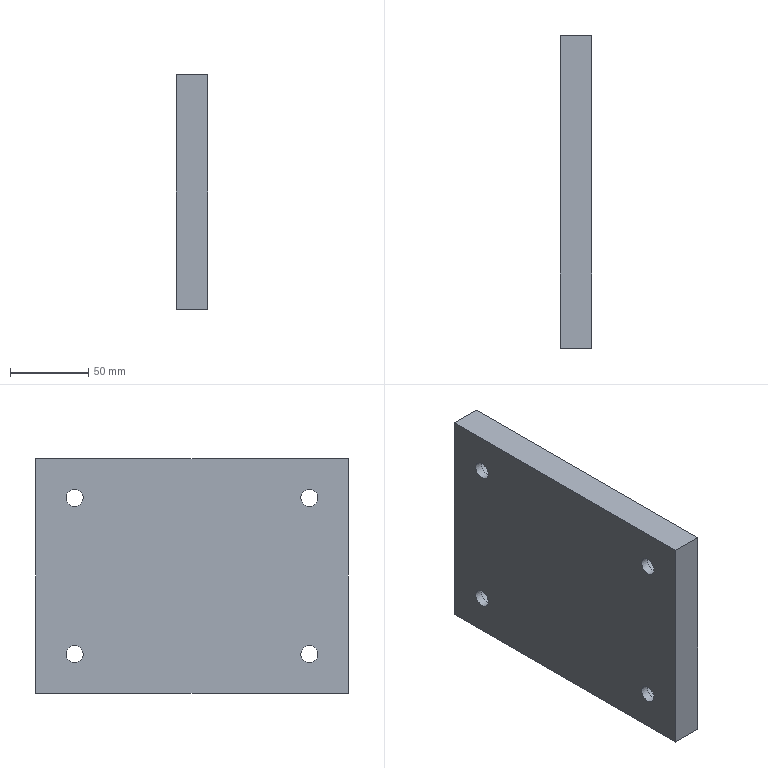Part | NX | features solid 2 | 1 solid | 18 faces | box 20 x 200 x 150 mm | volume 583668 mm3 | plane 10 | cylinder 8 | commonest cylinder face diameters 11 x4 17.5 x4
STEP:
#1=CARTESIAN_POINT('',(925.,225.,-376.25));
#2=VERTEX_POINT('',#1);
#3=CARTESIAN_POINT('',(925.,225.,-385.));
#4=DIRECTION('',(1.,0.,0.));
#5=DIRECTION('',(0.,0.,1.));
#6=AXIS2_PLACEMENT_3D('',#3,#4,#5);
#7=CIRCLE('',#6,8.75);
#8=EDGE_CURVE('',#2,#2,#7,.F.);
#9=ORIENTED_EDGE('',*,*,#8,.T.);
#10=EDGE_LOOP('',(#9));
#11=FACE_BOUND('',#10,.T.);
#12=CARTESIAN_POINT('',(925.,200.,-410.));
#13=VERTEX_POINT('',#12);
#14=CARTESIAN_POINT('',(925.,200.,-260.));
#15=VERTEX_POINT('',#14);
#16=CARTESIAN_POINT('',(925.,200.,-410.));
#17=DIRECTION('',(0.,0.,1.));
#18=VECTOR('',#17,1000.);
#19=LINE('',#16,#18);
#20=EDGE_CURVE('',#13,#15,#19,.T.);
#21=ORIENTED_EDGE('',*,*,#20,.F.);
#22=CARTESIAN_POINT('',(925.,400.,-410.));
#23=VERTEX_POINT('',#22);
#24=CARTESIAN_POINT('',(925.,300.,-410.));
#25=DIRECTION('',(0.,1.,0.));
#26=VECTOR('',#25,1000.);
#27=LINE('',#24,#26);
#28=EDGE_CURVE('',#13,#23,#27,.T.);
#29=ORIENTED_EDGE('',*,*,#28,.T.);
#30=CARTESIAN_POINT('',(925.,400.,-260.));
#31=VERTEX_POINT('',#30);
#32=CARTESIAN_POINT('',(925.,400.,-410.));
#33=DIRECTION('',(0.,0.,1.));
#34=VECTOR('',#33,1000.);
#35=LINE('',#32,#34);
#36=EDGE_CURVE('',#23,#31,#35,.T.);
#37=ORIENTED_EDGE('',*,*,#36,.T.);
#38=CARTESIAN_POINT('',(925.,300.,-260.));
#39=DIRECTION('',(0.,-1.,0.));
#40=VECTOR('',#39,1000.);
#41=LINE('',#38,#40);
#42=EDGE_CURVE('',#31,#15,#41,.T.);
#43=ORIENTED_EDGE('',*,*,#42,.T.);
#44=EDGE_LOOP('',(#21,#29,#37,#43));
#45=FACE_BOUND('',#44,.T.);
#46=CARTESIAN_POINT('',(925.,375.,-276.25));
#47=VERTEX_POINT('',#46);
#48=CARTESIAN_POINT('',(925.,375.,-285.));
#49=DIRECTION('',(-1.,0.,0.));
#50=DIRECTION('',(0.,0.,1.));
#51=AXIS2_PLACEMENT_3D('',#48,#49,#50);
#52=CIRCLE('',#51,8.75);
#53=EDGE_CURVE('',#47,#47,#52,.T.);
#54=ORIENTED_EDGE('',*,*,#53,.T.);
#55=EDGE_LOOP('',(#54));
#56=FACE_BOUND('',#55,.T.);
#57=CARTESIAN_POINT('',(925.,375.,-376.25));
#58=VERTEX_POINT('',#57);
#59=CARTESIAN_POINT('',(925.,375.,-385.));
#60=DIRECTION('',(-1.,0.,0.));
#61=DIRECTION('',(0.,0.,1.));
#62=AXIS2_PLACEMENT_3D('',#59,#60,#61);
#63=CIRCLE('',#62,8.75);
#64=EDGE_CURVE('',#58,#58,#63,.T.);
#65=ORIENTED_EDGE('',*,*,#64,.T.);
#66=EDGE_LOOP('',(#65));
#67=FACE_BOUND('',#66,.T.);
#68=CARTESIAN_POINT('',(925.,225.,-276.25));
#69=VERTEX_POINT('',#68);
#70=CARTESIAN_POINT('',(925.,225.,-285.));
#71=DIRECTION('',(1.,0.,0.));
#72=DIRECTION('',(0.,0.,1.));
#73=AXIS2_PLACEMENT_3D('',#70,#71,#72);
#74=CIRCLE('',#73,8.75);
#75=EDGE_CURVE('',#69,#69,#74,.F.);
#76=ORIENTED_EDGE('',*,*,#75,.T.);
#77=EDGE_LOOP('',(#76));
#78=FACE_BOUND('',#77,.T.);
#79=CARTESIAN_POINT('',(925.,300.,-410.));
#80=DIRECTION('',(1.,0.,0.));
#81=DIRECTION('',(0.,0.,-1.));
#82=AXIS2_PLACEMENT_3D('',#79,#80,#81);
#83=PLANE('',#82);
#84=ADVANCED_FACE('',(#11,#45,#56,#67,#78),#83,.T.);
#85=CARTESIAN_POINT('',(905.,400.,-260.));
#86=VERTEX_POINT('',#85);
#87=CARTESIAN_POINT('',(915.,400.,-260.));
#88=DIRECTION('',(1.,0.,0.));
#89=VECTOR('',#88,1000.);
#90=LINE('',#87,#89);
#91=EDGE_CURVE('',#86,#31,#90,.T.);
#92=ORIENTED_EDGE('',*,*,#91,.T.);
#93=ORIENTED_EDGE('',*,*,#36,.F.);
#94=CARTESIAN_POINT('',(905.,400.,-410.));
#95=VERTEX_POINT('',#94);
#96=CARTESIAN_POINT('',(915.,400.,-410.));
#97=DIRECTION('',(-1.,0.,0.));
#98=VECTOR('',#97,1000.);
#99=LINE('',#96,#98);
#100=EDGE_CURVE('',#23,#95,#99,.T.);
#101=ORIENTED_EDGE('',*,*,#100,.T.);
#102=CARTESIAN_POINT('',(905.,400.,-410.));
#103=DIRECTION('',(0.,0.,1.));
#104=VECTOR('',#103,1000.);
#105=LINE('',#102,#104);
#106=EDGE_CURVE('',#95,#86,#105,.T.);
#107=ORIENTED_EDGE('',*,*,#106,.T.);
#108=EDGE_LOOP('',(#92,#93,#101,#107));
#109=FACE_BOUND('',#108,.T.);
#110=CARTESIAN_POINT('',(915.,400.,-410.));
#111=DIRECTION('',(0.,1.,0.));
#112=DIRECTION('',(0.,0.,-1.));
#113=AXIS2_PLACEMENT_3D('',#110,#111,#112);
#114=PLANE('',#113);
#115=ADVANCED_FACE('',(#109),#114,.T.);
#116=CARTESIAN_POINT('',(905.,225.,-390.5));
#117=VERTEX_POINT('',#116);
#118=CARTESIAN_POINT('',(905.,225.,-385.));
#119=DIRECTION('',(-1.,0.,0.));
#120=DIRECTION('',(0.,0.,-1.));
#121=AXIS2_PLACEMENT_3D('',#118,#119,#120);
#122=CIRCLE('',#121,5.5);
#123=EDGE_CURVE('',#117,#117,#122,.T.);
#124=ORIENTED_EDGE('',*,*,#123,.F.);
#125=EDGE_LOOP('',(#124));
#126=FACE_BOUND('',#125,.T.);
#127=CARTESIAN_POINT('',(905.,225.,-290.5));
#128=VERTEX_POINT('',#127);
#129=CARTESIAN_POINT('',(905.,225.,-285.));
#130=DIRECTION('',(-1.,0.,0.));
#131=DIRECTION('',(0.,0.,-1.));
#132=AXIS2_PLACEMENT_3D('',#129,#130,#131);
#133=CIRCLE('',#132,5.5);
#134=EDGE_CURVE('',#128,#128,#133,.T.);
#135=ORIENTED_EDGE('',*,*,#134,.F.);
#136=EDGE_LOOP('',(#135));
#137=FACE_BOUND('',#136,.T.);
#138=CARTESIAN_POINT('',(905.,200.,-260.));
#139=VERTEX_POINT('',#138);
#140=CARTESIAN_POINT('',(905.,200.,-410.));
#141=VERTEX_POINT('',#140);
#142=CARTESIAN_POINT('',(905.,200.,-410.));
#143=DIRECTION('',(0.,0.,-1.));
#144=VECTOR('',#143,1000.);
#145=LINE('',#142,#144);
#146=EDGE_CURVE('',#139,#141,#145,.T.);
#147=ORIENTED_EDGE('',*,*,#146,.F.);
#148=CARTESIAN_POINT('',(905.,300.,-260.));
#149=DIRECTION('',(0.,1.,0.));
#150=VECTOR('',#149,1000.);
#151=LINE('',#148,#150);
#152=EDGE_CURVE('',#139,#86,#151,.T.);
#153=ORIENTED_EDGE('',*,*,#152,.T.);
#154=ORIENTED_EDGE('',*,*,#106,.F.);
#155=CARTESIAN_POINT('',(905.,300.,-410.));
#156=DIRECTION('',(0.,-1.,0.));
#157=VECTOR('',#156,1000.);
#158=LINE('',#155,#157);
#159=EDGE_CURVE('',#95,#141,#158,.T.);
#160=ORIENTED_EDGE('',*,*,#159,.T.);
#161=EDGE_LOOP('',(#147,#153,#154,#160));
#162=FACE_BOUND('',#161,.T.);
#163=CARTESIAN_POINT('',(905.,375.,-290.5));
#164=VERTEX_POINT('',#163);
#165=CARTESIAN_POINT('',(905.,375.,-285.));
#166=DIRECTION('',(1.,0.,0.));
#167=DIRECTION('',(0.,0.,-1.));
#168=AXIS2_PLACEMENT_3D('',#165,#166,#167);
#169=CIRCLE('',#168,5.5);
#170=EDGE_CURVE('',#164,#164,#169,.T.);
#171=ORIENTED_EDGE('',*,*,#170,.T.);
#172=EDGE_LOOP('',(#171));
#173=FACE_BOUND('',#172,.T.);
#174=CARTESIAN_POINT('',(905.,375.,-390.5));
#175=VERTEX_POINT('',#174);
#176=CARTESIAN_POINT('',(905.,375.,-385.));
#177=DIRECTION('',(1.,0.,0.));
#178=DIRECTION('',(0.,0.,-1.));
#179=AXIS2_PLACEMENT_3D('',#176,#177,#178);
#180=CIRCLE('',#179,5.5);
#181=EDGE_CURVE('',#175,#175,#180,.T.);
#182=ORIENTED_EDGE('',*,*,#181,.T.);
#183=EDGE_LOOP('',(#182));
#184=FACE_BOUND('',#183,.T.);
#185=CARTESIAN_POINT('',(905.,300.,-410.));
#186=DIRECTION('',(-1.,0.,0.));
#187=DIRECTION('',(0.,0.,1.));
#188=AXIS2_PLACEMENT_3D('',#185,#186,#187);
#189=PLANE('',#188);
#190=ADVANCED_FACE('',(#126,#137,#162,#173,#184),#189,.T.);
#191=CARTESIAN_POINT('',(910.,375.,-293.75));
#192=VERTEX_POINT('',#191);
#193=CARTESIAN_POINT('',(910.,375.,-285.));
#194=DIRECTION('',(1.,0.,0.));
#195=DIRECTION('',(0.,0.,-1.));
#196=AXIS2_PLACEMENT_3D('',#193,#194,#195);
#197=CIRCLE('',#196,8.75);
#198=EDGE_CURVE('',#192,#192,#197,.T.);
#199=ORIENTED_EDGE('',*,*,#198,.T.);
#200=EDGE_LOOP('',(#199));
#201=FACE_BOUND('',#200,.T.);
#202=CARTESIAN_POINT('',(910.,375.,-279.5));
#203=VERTEX_POINT('',#202);
#204=CARTESIAN_POINT('',(910.,375.,-285.));
#205=DIRECTION('',(-1.,0.,0.));
#206=DIRECTION('',(0.,0.,1.));
#207=AXIS2_PLACEMENT_3D('',#204,#205,#206);
#208=CIRCLE('',#207,5.5);
#209=EDGE_CURVE('',#203,#203,#208,.F.);
#210=ORIENTED_EDGE('',*,*,#209,.F.);
#211=EDGE_LOOP('',(#210));
#212=FACE_BOUND('',#211,.T.);
#213=CARTESIAN_POINT('',(910.,375.,-285.));
#214=DIRECTION('',(-1.,0.,0.));
#215=DIRECTION('',(0.,0.,1.));
#216=AXIS2_PLACEMENT_3D('',#213,#214,#215);
#217=PLANE('',#216);
#218=ADVANCED_FACE('',(#201,#212),#217,.F.);
#219=ORIENTED_EDGE('',*,*,#209,.T.);
#220=EDGE_LOOP('',(#219));
#221=FACE_BOUND('',#220,.T.);
#222=ORIENTED_EDGE('',*,*,#170,.F.);
#223=EDGE_LOOP('',(#222));
#224=FACE_BOUND('',#223,.T.);
#225=CARTESIAN_POINT('',(905.,375.,-285.));
#226=DIRECTION('',(1.,0.,0.));
#227=DIRECTION('',(0.,0.,-1.));
#228=AXIS2_PLACEMENT_3D('',#225,#226,#227);
#229=CYLINDRICAL_SURFACE('',#228,5.5);
#230=ADVANCED_FACE('',(#221,#224),#229,.F.);
#231=CARTESIAN_POINT('',(915.,200.,-260.));
#232=DIRECTION('',(-1.,0.,0.));
#233=VECTOR('',#232,1000.);
#234=LINE('',#231,#233);
#235=EDGE_CURVE('',#15,#139,#234,.T.);
#236=ORIENTED_EDGE('',*,*,#235,.F.);
#237=ORIENTED_EDGE('',*,*,#42,.F.);
#238=ORIENTED_EDGE('',*,*,#91,.F.);
#239=ORIENTED_EDGE('',*,*,#152,.F.);
#240=EDGE_LOOP('',(#236,#237,#238,#239));
#241=FACE_BOUND('',#240,.T.);
#242=CARTESIAN_POINT('',(915.,300.,-260.));
#243=DIRECTION('',(0.,0.,1.));
#244=DIRECTION('',(0.,1.,0.));
#245=AXIS2_PLACEMENT_3D('',#242,#243,#244);
#246=PLANE('',#245);
#247=ADVANCED_FACE('',(#241),#246,.T.);
#248=ORIENTED_EDGE('',*,*,#53,.F.);
#249=EDGE_LOOP('',(#248));
#250=FACE_BOUND('',#249,.T.);
#251=ORIENTED_EDGE('',*,*,#198,.F.);
#252=EDGE_LOOP('',(#251));
#253=FACE_BOUND('',#252,.T.);
#254=CARTESIAN_POINT('',(910.,375.,-285.));
#255=DIRECTION('',(1.,0.,0.));
#256=DIRECTION('',(0.,0.,-1.));
#257=AXIS2_PLACEMENT_3D('',#254,#255,#256);
#258=CYLINDRICAL_SURFACE('',#257,8.75);
#259=ADVANCED_FACE('',(#250,#253),#258,.F.);
#260=CARTESIAN_POINT('',(910.,375.,-393.75));
#261=VERTEX_POINT('',#260);
#262=CARTESIAN_POINT('',(910.,375.,-385.));
#263=DIRECTION('',(1.,0.,0.));
#264=DIRECTION('',(0.,0.,-1.));
#265=AXIS2_PLACEMENT_3D('',#262,#263,#264);
#266=CIRCLE('',#265,8.75);
#267=EDGE_CURVE('',#261,#261,#266,.T.);
#268=ORIENTED_EDGE('',*,*,#267,.T.);
#269=EDGE_LOOP('',(#268));
#270=FACE_BOUND('',#269,.T.);
#271=CARTESIAN_POINT('',(910.,375.,-379.5));
#272=VERTEX_POINT('',#271);
#273=CARTESIAN_POINT('',(910.,375.,-385.));
#274=DIRECTION('',(-1.,0.,0.));
#275=DIRECTION('',(0.,0.,1.));
#276=AXIS2_PLACEMENT_3D('',#273,#274,#275);
#277=CIRCLE('',#276,5.5);
#278=EDGE_CURVE('',#272,#272,#277,.F.);
#279=ORIENTED_EDGE('',*,*,#278,.F.);
#280=EDGE_LOOP('',(#279));
#281=FACE_BOUND('',#280,.T.);
#282=CARTESIAN_POINT('',(910.,375.,-310.));
#283=DIRECTION('',(-1.,0.,0.));
#284=DIRECTION('',(0.,0.,1.));
#285=AXIS2_PLACEMENT_3D('',#282,#283,#284);
#286=PLANE('',#285);
#287=ADVANCED_FACE('',(#270,#281),#286,.F.);
#288=ORIENTED_EDGE('',*,*,#278,.T.);
#289=EDGE_LOOP('',(#288));
#290=FACE_BOUND('',#289,.T.);
#291=ORIENTED_EDGE('',*,*,#181,.F.);
#292=EDGE_LOOP('',(#291));
#293=FACE_BOUND('',#292,.T.);
#294=CARTESIAN_POINT('',(905.,375.,-385.));
#295=DIRECTION('',(1.,0.,0.));
#296=DIRECTION('',(0.,0.,-1.));
#297=AXIS2_PLACEMENT_3D('',#294,#295,#296);
#298=CYLINDRICAL_SURFACE('',#297,5.5);
#299=ADVANCED_FACE('',(#290,#293),#298,.F.);
#300=CARTESIAN_POINT('',(915.,200.,-410.));
#301=DIRECTION('',(1.,0.,0.));
#302=VECTOR('',#301,1000.);
#303=LINE('',#300,#302);
#304=EDGE_CURVE('',#141,#13,#303,.T.);
#305=ORIENTED_EDGE('',*,*,#304,.F.);
#306=ORIENTED_EDGE('',*,*,#159,.F.);
#307=ORIENTED_EDGE('',*,*,#100,.F.);
#308=ORIENTED_EDGE('',*,*,#28,.F.);
#309=EDGE_LOOP('',(#305,#306,#307,#308));
#310=FACE_BOUND('',#309,.T.);
#311=CARTESIAN_POINT('',(915.,300.,-410.));
#312=DIRECTION('',(0.,0.,-1.));
#313=DIRECTION('',(0.,-1.,0.));
#314=AXIS2_PLACEMENT_3D('',#311,#312,#313);
#315=PLANE('',#314);
#316=ADVANCED_FACE('',(#310),#315,.T.);
#317=ORIENTED_EDGE('',*,*,#64,.F.);
#318=EDGE_LOOP('',(#317));
#319=FACE_BOUND('',#318,.T.);
#320=ORIENTED_EDGE('',*,*,#267,.F.);
#321=EDGE_LOOP('',(#320));
#322=FACE_BOUND('',#321,.T.);
#323=CARTESIAN_POINT('',(910.,375.,-385.));
#324=DIRECTION('',(1.,0.,0.));
#325=DIRECTION('',(0.,0.,-1.));
#326=AXIS2_PLACEMENT_3D('',#323,#324,#325);
#327=CYLINDRICAL_SURFACE('',#326,8.75);
#328=ADVANCED_FACE('',(#319,#322),#327,.F.);
#329=ORIENTED_EDGE('',*,*,#235,.T.);
#330=ORIENTED_EDGE('',*,*,#146,.T.);
#331=ORIENTED_EDGE('',*,*,#304,.T.);
#332=ORIENTED_EDGE('',*,*,#20,.T.);
#333=EDGE_LOOP('',(#329,#330,#331,#332));
#334=FACE_BOUND('',#333,.T.);
#335=CARTESIAN_POINT('',(915.,200.,-335.));
#336=DIRECTION('',(0.,1.,0.));
#337=DIRECTION('',(0.,0.,-1.));
#338=AXIS2_PLACEMENT_3D('',#335,#336,#337);
#339=PLANE('',#338);
#340=ADVANCED_FACE('',(#334),#339,.F.);
#341=ORIENTED_EDGE('',*,*,#8,.F.);
#342=EDGE_LOOP('',(#341));
#343=FACE_BOUND('',#342,.T.);
#344=CARTESIAN_POINT('',(910.,225.,-393.75));
#345=VERTEX_POINT('',#344);
#346=CARTESIAN_POINT('',(910.,225.,-385.));
#347=DIRECTION('',(1.,0.,0.));
#348=DIRECTION('',(0.,0.,-1.));
#349=AXIS2_PLACEMENT_3D('',#346,#347,#348);
#350=CIRCLE('',#349,8.75);
#351=EDGE_CURVE('',#345,#345,#350,.T.);
#352=ORIENTED_EDGE('',*,*,#351,.F.);
#353=EDGE_LOOP('',(#352));
#354=FACE_BOUND('',#353,.T.);
#355=CARTESIAN_POINT('',(960.,225.,-385.));
#356=DIRECTION('',(-1.,0.,0.));
#357=DIRECTION('',(0.,0.,-1.));
#358=AXIS2_PLACEMENT_3D('',#355,#356,#357);
#359=CYLINDRICAL_SURFACE('',#358,8.75);
#360=ADVANCED_FACE('',(#343,#354),#359,.F.);
#361=CARTESIAN_POINT('',(910.,225.,-379.5));
#362=VERTEX_POINT('',#361);
#363=CARTESIAN_POINT('',(910.,225.,-385.));
#364=DIRECTION('',(1.,0.,0.));
#365=DIRECTION('',(0.,0.,1.));
#366=AXIS2_PLACEMENT_3D('',#363,#364,#365);
#367=CIRCLE('',#366,5.5);
#368=EDGE_CURVE('',#362,#362,#367,.T.);
#369=ORIENTED_EDGE('',*,*,#368,.F.);
#370=EDGE_LOOP('',(#369));
#371=FACE_BOUND('',#370,.T.);
#372=ORIENTED_EDGE('',*,*,#351,.T.);
#373=EDGE_LOOP('',(#372));
#374=FACE_BOUND('',#373,.T.);
#375=CARTESIAN_POINT('',(910.,225.,-385.));
#376=DIRECTION('',(1.,0.,0.));
#377=DIRECTION('',(0.,0.,1.));
#378=AXIS2_PLACEMENT_3D('',#375,#376,#377);
#379=PLANE('',#378);
#380=ADVANCED_FACE('',(#371,#374),#379,.T.);
#381=ORIENTED_EDGE('',*,*,#75,.F.);
#382=EDGE_LOOP('',(#381));
#383=FACE_BOUND('',#382,.T.);
#384=CARTESIAN_POINT('',(910.,225.,-293.75));
#385=VERTEX_POINT('',#384);
#386=CARTESIAN_POINT('',(910.,225.,-285.));
#387=DIRECTION('',(1.,0.,0.));
#388=DIRECTION('',(0.,0.,-1.));
#389=AXIS2_PLACEMENT_3D('',#386,#387,#388);
#390=CIRCLE('',#389,8.75);
#391=EDGE_CURVE('',#385,#385,#390,.T.);
#392=ORIENTED_EDGE('',*,*,#391,.F.);
#393=EDGE_LOOP('',(#392));
#394=FACE_BOUND('',#393,.T.);
#395=CARTESIAN_POINT('',(960.,225.,-285.));
#396=DIRECTION('',(-1.,0.,0.));
#397=DIRECTION('',(0.,0.,-1.));
#398=AXIS2_PLACEMENT_3D('',#395,#396,#397);
#399=CYLINDRICAL_SURFACE('',#398,8.75);
#400=ADVANCED_FACE('',(#383,#394),#399,.F.);
#401=CARTESIAN_POINT('',(910.,225.,-279.5));
#402=VERTEX_POINT('',#401);
#403=CARTESIAN_POINT('',(910.,225.,-285.));
#404=DIRECTION('',(1.,0.,0.));
#405=DIRECTION('',(0.,0.,1.));
#406=AXIS2_PLACEMENT_3D('',#403,#404,#405);
#407=CIRCLE('',#406,5.5);
#408=EDGE_CURVE('',#402,#402,#407,.T.);
#409=ORIENTED_EDGE('',*,*,#408,.F.);
#410=EDGE_LOOP('',(#409));
#411=FACE_BOUND('',#410,.T.);
#412=ORIENTED_EDGE('',*,*,#391,.T.);
#413=EDGE_LOOP('',(#412));
#414=FACE_BOUND('',#413,.T.);
#415=CARTESIAN_POINT('',(910.,225.,-285.));
#416=DIRECTION('',(1.,0.,0.));
#417=DIRECTION('',(0.,0.,1.));
#418=AXIS2_PLACEMENT_3D('',#415,#416,#417);
#419=PLANE('',#418);
#420=ADVANCED_FACE('',(#411,#414),#419,.T.);
#421=ORIENTED_EDGE('',*,*,#134,.T.);
#422=EDGE_LOOP('',(#421));
#423=FACE_BOUND('',#422,.T.);
#424=ORIENTED_EDGE('',*,*,#408,.T.);
#425=EDGE_LOOP('',(#424));
#426=FACE_BOUND('',#425,.T.);
#427=CARTESIAN_POINT('',(860.,225.,-285.));
#428=DIRECTION('',(1.,0.,0.));
#429=DIRECTION('',(0.,0.,1.));
#430=AXIS2_PLACEMENT_3D('',#427,#428,#429);
#431=CYLINDRICAL_SURFACE('',#430,5.5);
#432=ADVANCED_FACE('',(#423,#426),#431,.F.);
#433=ORIENTED_EDGE('',*,*,#123,.T.);
#434=EDGE_LOOP('',(#433));
#435=FACE_BOUND('',#434,.T.);
#436=ORIENTED_EDGE('',*,*,#368,.T.);
#437=EDGE_LOOP('',(#436));
#438=FACE_BOUND('',#437,.T.);
#439=CARTESIAN_POINT('',(860.,225.,-385.));
#440=DIRECTION('',(1.,0.,0.));
#441=DIRECTION('',(0.,0.,1.));
#442=AXIS2_PLACEMENT_3D('',#439,#440,#441);
#443=CYLINDRICAL_SURFACE('',#442,5.5);
#444=ADVANCED_FACE('',(#435,#438),#443,.F.);
#445=CLOSED_SHELL('',(#84,#115,#190,#218,#230,#247,#259,#287,#299,#316,#328,#340,#360,#380,#400,#420,#432,#444));
#446=MANIFOLD_SOLID_BREP('',#445);
#447=(LENGTH_UNIT()NAMED_UNIT(*)SI_UNIT(.MILLI.,.METRE.));
#448=UNCERTAINTY_MEASURE_WITH_UNIT(LENGTH_MEASURE(0.00001),#447,'','');
#449=(NAMED_UNIT(*)PLANE_ANGLE_UNIT()SI_UNIT($,.RADIAN.));
#450=(NAMED_UNIT(*)SI_UNIT($,.STERADIAN.)SOLID_ANGLE_UNIT());
#451=(GEOMETRIC_REPRESENTATION_CONTEXT(3)GLOBAL_UNCERTAINTY_ASSIGNED_CONTEXT((#448))GLOBAL_UNIT_ASSIGNED_CONTEXT((#447,#449,#450))REPRESENTATION_CONTEXT('',''));
#452=ADVANCED_BREP_SHAPE_REPRESENTATION('',(#446),#451);